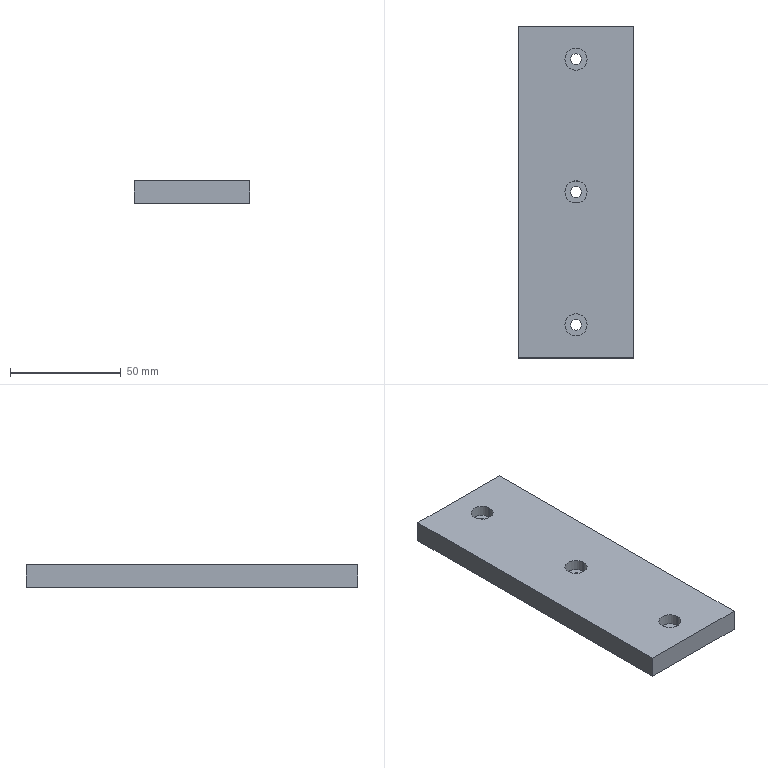Part | SolidWorks | features Chamfer 1, Extrusion 1, HoleWzd 1 | 1 solid | 21 faces | box 52 x 150 x 10 mm | volume 76527 mm3 | cylinder 12 | plane 9 | commonest cylinder face diameters 5 x6 10 x6
STEP:
#1=CARTESIAN_POINT('',(-5.,60.,0.));
#2=VERTEX_POINT('',#1);
#3=CARTESIAN_POINT('',(5.,60.,0.));
#4=VERTEX_POINT('',#3);
#5=CARTESIAN_POINT('',(0.,60.,0.));
#6=DIRECTION('',(0.,0.,1.));
#7=DIRECTION('',(1.,0.,0.));
#8=AXIS2_PLACEMENT_3D('',#5,#6,#7);
#9=CIRCLE('',#8,5.);
#10=EDGE_CURVE('',#2,#4,#9,.T.);
#11=ORIENTED_EDGE('',*,*,#10,.F.);
#12=CARTESIAN_POINT('',(-5.,60.,5.));
#13=VERTEX_POINT('',#12);
#14=CARTESIAN_POINT('',(-5.,60.,5.));
#15=DIRECTION('',(0.,0.,1.));
#16=VECTOR('',#15,1000.);
#17=LINE('',#14,#16);
#18=EDGE_CURVE('',#2,#13,#17,.T.);
#19=ORIENTED_EDGE('',*,*,#18,.T.);
#20=CARTESIAN_POINT('',(5.,60.,5.));
#21=VERTEX_POINT('',#20);
#22=CARTESIAN_POINT('',(0.,60.,5.));
#23=DIRECTION('',(0.,0.,1.));
#24=DIRECTION('',(1.,0.,0.));
#25=AXIS2_PLACEMENT_3D('',#22,#23,#24);
#26=CIRCLE('',#25,5.);
#27=EDGE_CURVE('',#13,#21,#26,.T.);
#28=ORIENTED_EDGE('',*,*,#27,.T.);
#29=CARTESIAN_POINT('',(5.,60.,5.));
#30=DIRECTION('',(0.,0.,1.));
#31=VECTOR('',#30,1000.);
#32=LINE('',#29,#31);
#33=EDGE_CURVE('',#4,#21,#32,.T.);
#34=ORIENTED_EDGE('',*,*,#33,.F.);
#35=EDGE_LOOP('',(#11,#19,#28,#34));
#36=FACE_OUTER_BOUND('',#35,.T.);
#37=CARTESIAN_POINT('',(0.,60.,5.));
#38=DIRECTION('',(0.,0.,1.));
#39=DIRECTION('',(1.,0.,0.));
#40=AXIS2_PLACEMENT_3D('',#37,#38,#39);
#41=CYLINDRICAL_SURFACE('',#40,5.);
#42=ADVANCED_FACE('',(#36),#41,.F.);
#43=CARTESIAN_POINT('',(-2.5,60.,-5.));
#44=VERTEX_POINT('',#43);
#45=CARTESIAN_POINT('',(2.5,60.,-5.));
#46=VERTEX_POINT('',#45);
#47=CARTESIAN_POINT('',(0.,60.,-5.));
#48=DIRECTION('',(0.,0.,1.));
#49=DIRECTION('',(1.,0.,0.));
#50=AXIS2_PLACEMENT_3D('',#47,#48,#49);
#51=CIRCLE('',#50,2.5);
#52=EDGE_CURVE('',#44,#46,#51,.T.);
#53=ORIENTED_EDGE('',*,*,#52,.F.);
#54=CARTESIAN_POINT('',(-2.5,60.,0.));
#55=VERTEX_POINT('',#54);
#56=CARTESIAN_POINT('',(-2.5,60.,5.));
#57=DIRECTION('',(0.,0.,1.));
#58=VECTOR('',#57,1000.);
#59=LINE('',#56,#58);
#60=EDGE_CURVE('',#44,#55,#59,.T.);
#61=ORIENTED_EDGE('',*,*,#60,.T.);
#62=CARTESIAN_POINT('',(2.5,60.,0.));
#63=VERTEX_POINT('',#62);
#64=CARTESIAN_POINT('',(0.,60.,0.));
#65=DIRECTION('',(0.,0.,1.));
#66=DIRECTION('',(1.,0.,0.));
#67=AXIS2_PLACEMENT_3D('',#64,#65,#66);
#68=CIRCLE('',#67,2.5);
#69=EDGE_CURVE('',#55,#63,#68,.T.);
#70=ORIENTED_EDGE('',*,*,#69,.T.);
#71=CARTESIAN_POINT('',(2.5,60.,5.));
#72=DIRECTION('',(0.,0.,1.));
#73=VECTOR('',#72,1000.);
#74=LINE('',#71,#73);
#75=EDGE_CURVE('',#46,#63,#74,.T.);
#76=ORIENTED_EDGE('',*,*,#75,.F.);
#77=EDGE_LOOP('',(#53,#61,#70,#76));
#78=FACE_OUTER_BOUND('',#77,.T.);
#79=CARTESIAN_POINT('',(0.,60.,5.));
#80=DIRECTION('',(0.,0.,1.));
#81=DIRECTION('',(1.,0.,0.));
#82=AXIS2_PLACEMENT_3D('',#79,#80,#81);
#83=CYLINDRICAL_SURFACE('',#82,2.5);
#84=ADVANCED_FACE('',(#78),#83,.F.);
#85=CARTESIAN_POINT('',(-5.,-60.,0.));
#86=VERTEX_POINT('',#85);
#87=CARTESIAN_POINT('',(5.,-60.,0.));
#88=VERTEX_POINT('',#87);
#89=CARTESIAN_POINT('',(0.,-60.,0.));
#90=DIRECTION('',(0.,0.,1.));
#91=DIRECTION('',(1.,0.,0.));
#92=AXIS2_PLACEMENT_3D('',#89,#90,#91);
#93=CIRCLE('',#92,5.);
#94=EDGE_CURVE('',#86,#88,#93,.T.);
#95=ORIENTED_EDGE('',*,*,#94,.F.);
#96=CARTESIAN_POINT('',(-5.,-60.,5.));
#97=VERTEX_POINT('',#96);
#98=CARTESIAN_POINT('',(-5.,-60.,5.));
#99=DIRECTION('',(0.,0.,1.));
#100=VECTOR('',#99,1000.);
#101=LINE('',#98,#100);
#102=EDGE_CURVE('',#86,#97,#101,.T.);
#103=ORIENTED_EDGE('',*,*,#102,.T.);
#104=CARTESIAN_POINT('',(5.,-60.,5.));
#105=VERTEX_POINT('',#104);
#106=CARTESIAN_POINT('',(0.,-60.,5.));
#107=DIRECTION('',(0.,0.,1.));
#108=DIRECTION('',(1.,0.,0.));
#109=AXIS2_PLACEMENT_3D('',#106,#107,#108);
#110=CIRCLE('',#109,5.);
#111=EDGE_CURVE('',#97,#105,#110,.T.);
#112=ORIENTED_EDGE('',*,*,#111,.T.);
#113=CARTESIAN_POINT('',(5.,-60.,5.));
#114=DIRECTION('',(0.,0.,1.));
#115=VECTOR('',#114,1000.);
#116=LINE('',#113,#115);
#117=EDGE_CURVE('',#88,#105,#116,.T.);
#118=ORIENTED_EDGE('',*,*,#117,.F.);
#119=EDGE_LOOP('',(#95,#103,#112,#118));
#120=FACE_OUTER_BOUND('',#119,.T.);
#121=CARTESIAN_POINT('',(0.,-60.,5.));
#122=DIRECTION('',(0.,0.,1.));
#123=DIRECTION('',(1.,0.,0.));
#124=AXIS2_PLACEMENT_3D('',#121,#122,#123);
#125=CYLINDRICAL_SURFACE('',#124,5.);
#126=ADVANCED_FACE('',(#120),#125,.F.);
#127=CARTESIAN_POINT('',(-2.5,-60.,-5.));
#128=VERTEX_POINT('',#127);
#129=CARTESIAN_POINT('',(2.5,-60.,-5.));
#130=VERTEX_POINT('',#129);
#131=CARTESIAN_POINT('',(0.,-60.,-5.));
#132=DIRECTION('',(0.,0.,1.));
#133=DIRECTION('',(1.,0.,0.));
#134=AXIS2_PLACEMENT_3D('',#131,#132,#133);
#135=CIRCLE('',#134,2.5);
#136=EDGE_CURVE('',#128,#130,#135,.T.);
#137=ORIENTED_EDGE('',*,*,#136,.F.);
#138=CARTESIAN_POINT('',(-2.5,-60.,0.));
#139=VERTEX_POINT('',#138);
#140=CARTESIAN_POINT('',(-2.5,-60.,5.));
#141=DIRECTION('',(0.,0.,1.));
#142=VECTOR('',#141,1000.);
#143=LINE('',#140,#142);
#144=EDGE_CURVE('',#128,#139,#143,.T.);
#145=ORIENTED_EDGE('',*,*,#144,.T.);
#146=CARTESIAN_POINT('',(2.5,-60.,0.));
#147=VERTEX_POINT('',#146);
#148=CARTESIAN_POINT('',(0.,-60.,0.));
#149=DIRECTION('',(0.,0.,1.));
#150=DIRECTION('',(1.,0.,0.));
#151=AXIS2_PLACEMENT_3D('',#148,#149,#150);
#152=CIRCLE('',#151,2.5);
#153=EDGE_CURVE('',#139,#147,#152,.T.);
#154=ORIENTED_EDGE('',*,*,#153,.T.);
#155=CARTESIAN_POINT('',(2.5,-60.,5.));
#156=DIRECTION('',(0.,0.,1.));
#157=VECTOR('',#156,1000.);
#158=LINE('',#155,#157);
#159=EDGE_CURVE('',#130,#147,#158,.T.);
#160=ORIENTED_EDGE('',*,*,#159,.F.);
#161=EDGE_LOOP('',(#137,#145,#154,#160));
#162=FACE_OUTER_BOUND('',#161,.T.);
#163=CARTESIAN_POINT('',(0.,-60.,5.));
#164=DIRECTION('',(0.,0.,1.));
#165=DIRECTION('',(1.,0.,0.));
#166=AXIS2_PLACEMENT_3D('',#163,#164,#165);
#167=CYLINDRICAL_SURFACE('',#166,2.5);
#168=ADVANCED_FACE('',(#162),#167,.F.);
#169=CARTESIAN_POINT('',(-5.,0.,0.));
#170=VERTEX_POINT('',#169);
#171=CARTESIAN_POINT('',(5.,0.,0.));
#172=VERTEX_POINT('',#171);
#173=CARTESIAN_POINT('',(0.,0.,0.));
#174=DIRECTION('',(0.,0.,1.));
#175=DIRECTION('',(1.,0.,0.));
#176=AXIS2_PLACEMENT_3D('',#173,#174,#175);
#177=CIRCLE('',#176,5.);
#178=EDGE_CURVE('',#170,#172,#177,.T.);
#179=ORIENTED_EDGE('',*,*,#178,.F.);
#180=CARTESIAN_POINT('',(-5.,0.,5.));
#181=VERTEX_POINT('',#180);
#182=CARTESIAN_POINT('',(-5.,0.,5.));
#183=DIRECTION('',(0.,0.,1.));
#184=VECTOR('',#183,1000.);
#185=LINE('',#182,#184);
#186=EDGE_CURVE('',#170,#181,#185,.T.);
#187=ORIENTED_EDGE('',*,*,#186,.T.);
#188=CARTESIAN_POINT('',(5.,0.,5.));
#189=VERTEX_POINT('',#188);
#190=CARTESIAN_POINT('',(0.,0.,5.));
#191=DIRECTION('',(0.,0.,1.));
#192=DIRECTION('',(1.,0.,0.));
#193=AXIS2_PLACEMENT_3D('',#190,#191,#192);
#194=CIRCLE('',#193,5.);
#195=EDGE_CURVE('',#181,#189,#194,.T.);
#196=ORIENTED_EDGE('',*,*,#195,.T.);
#197=CARTESIAN_POINT('',(5.,0.,5.));
#198=DIRECTION('',(0.,0.,1.));
#199=VECTOR('',#198,1000.);
#200=LINE('',#197,#199);
#201=EDGE_CURVE('',#172,#189,#200,.T.);
#202=ORIENTED_EDGE('',*,*,#201,.F.);
#203=EDGE_LOOP('',(#179,#187,#196,#202));
#204=FACE_OUTER_BOUND('',#203,.T.);
#205=CARTESIAN_POINT('',(0.,0.,5.));
#206=DIRECTION('',(0.,0.,1.));
#207=DIRECTION('',(1.,0.,0.));
#208=AXIS2_PLACEMENT_3D('',#205,#206,#207);
#209=CYLINDRICAL_SURFACE('',#208,5.);
#210=ADVANCED_FACE('',(#204),#209,.F.);
#211=CARTESIAN_POINT('',(-2.5,0.,-5.));
#212=VERTEX_POINT('',#211);
#213=CARTESIAN_POINT('',(2.5,0.,-5.));
#214=VERTEX_POINT('',#213);
#215=CARTESIAN_POINT('',(0.,0.,-5.));
#216=DIRECTION('',(0.,0.,1.));
#217=DIRECTION('',(1.,0.,0.));
#218=AXIS2_PLACEMENT_3D('',#215,#216,#217);
#219=CIRCLE('',#218,2.5);
#220=EDGE_CURVE('',#212,#214,#219,.T.);
#221=ORIENTED_EDGE('',*,*,#220,.F.);
#222=CARTESIAN_POINT('',(-2.5,0.,0.));
#223=VERTEX_POINT('',#222);
#224=CARTESIAN_POINT('',(-2.5,0.,5.));
#225=DIRECTION('',(0.,0.,1.));
#226=VECTOR('',#225,1000.);
#227=LINE('',#224,#226);
#228=EDGE_CURVE('',#212,#223,#227,.T.);
#229=ORIENTED_EDGE('',*,*,#228,.T.);
#230=CARTESIAN_POINT('',(2.5,0.,0.));
#231=VERTEX_POINT('',#230);
#232=CARTESIAN_POINT('',(0.,0.,0.));
#233=DIRECTION('',(0.,0.,1.));
#234=DIRECTION('',(1.,0.,0.));
#235=AXIS2_PLACEMENT_3D('',#232,#233,#234);
#236=CIRCLE('',#235,2.5);
#237=EDGE_CURVE('',#223,#231,#236,.T.);
#238=ORIENTED_EDGE('',*,*,#237,.T.);
#239=CARTESIAN_POINT('',(2.5,0.,5.));
#240=DIRECTION('',(0.,0.,1.));
#241=VECTOR('',#240,1000.);
#242=LINE('',#239,#241);
#243=EDGE_CURVE('',#214,#231,#242,.T.);
#244=ORIENTED_EDGE('',*,*,#243,.F.);
#245=EDGE_LOOP('',(#221,#229,#238,#244));
#246=FACE_OUTER_BOUND('',#245,.T.);
#247=CARTESIAN_POINT('',(0.,0.,5.));
#248=DIRECTION('',(0.,0.,1.));
#249=DIRECTION('',(1.,0.,0.));
#250=AXIS2_PLACEMENT_3D('',#247,#248,#249);
#251=CYLINDRICAL_SURFACE('',#250,2.5);
#252=ADVANCED_FACE('',(#246),#251,.F.);
#253=CARTESIAN_POINT('',(-26.,75.,-5.));
#254=VERTEX_POINT('',#253);
#255=CARTESIAN_POINT('',(-26.,-75.,-5.));
#256=VERTEX_POINT('',#255);
#257=CARTESIAN_POINT('',(-26.,-75.,-5.));
#258=DIRECTION('',(0.,-1.,0.));
#259=VECTOR('',#258,1000.);
#260=LINE('',#257,#259);
#261=EDGE_CURVE('',#254,#256,#260,.T.);
#262=ORIENTED_EDGE('',*,*,#261,.T.);
#263=CARTESIAN_POINT('',(-26.,-75.,5.));
#264=VERTEX_POINT('',#263);
#265=CARTESIAN_POINT('',(-26.,-75.,5.));
#266=DIRECTION('',(0.,0.,-1.));
#267=VECTOR('',#266,1000.);
#268=LINE('',#265,#267);
#269=EDGE_CURVE('',#264,#256,#268,.T.);
#270=ORIENTED_EDGE('',*,*,#269,.F.);
#271=CARTESIAN_POINT('',(-26.,75.,5.));
#272=VERTEX_POINT('',#271);
#273=CARTESIAN_POINT('',(-26.,-75.,5.));
#274=DIRECTION('',(0.,-1.,0.));
#275=VECTOR('',#274,1000.);
#276=LINE('',#273,#275);
#277=EDGE_CURVE('',#272,#264,#276,.T.);
#278=ORIENTED_EDGE('',*,*,#277,.F.);
#279=CARTESIAN_POINT('',(-26.,75.,5.));
#280=DIRECTION('',(0.,0.,-1.));
#281=VECTOR('',#280,1000.);
#282=LINE('',#279,#281);
#283=EDGE_CURVE('',#272,#254,#282,.T.);
#284=ORIENTED_EDGE('',*,*,#283,.T.);
#285=EDGE_LOOP('',(#262,#270,#278,#284));
#286=FACE_OUTER_BOUND('',#285,.T.);
#287=CARTESIAN_POINT('',(-26.,-75.,5.));
#288=DIRECTION('',(1.,0.,0.));
#289=DIRECTION('',(0.,0.,-1.));
#290=AXIS2_PLACEMENT_3D('',#287,#288,#289);
#291=PLANE('',#290);
#292=ADVANCED_FACE('',(#286),#291,.F.);
#293=CARTESIAN_POINT('',(26.,-75.,-5.));
#294=VERTEX_POINT('',#293);
#295=CARTESIAN_POINT('',(26.,-75.,-5.));
#296=DIRECTION('',(1.,0.,0.));
#297=VECTOR('',#296,1000.);
#298=LINE('',#295,#297);
#299=EDGE_CURVE('',#256,#294,#298,.T.);
#300=ORIENTED_EDGE('',*,*,#299,.T.);
#301=CARTESIAN_POINT('',(26.,-75.,5.));
#302=VERTEX_POINT('',#301);
#303=CARTESIAN_POINT('',(26.,-75.,5.));
#304=DIRECTION('',(0.,0.,-1.));
#305=VECTOR('',#304,1000.);
#306=LINE('',#303,#305);
#307=EDGE_CURVE('',#302,#294,#306,.T.);
#308=ORIENTED_EDGE('',*,*,#307,.F.);
#309=CARTESIAN_POINT('',(26.,-75.,5.));
#310=DIRECTION('',(1.,0.,0.));
#311=VECTOR('',#310,1000.);
#312=LINE('',#309,#311);
#313=EDGE_CURVE('',#264,#302,#312,.T.);
#314=ORIENTED_EDGE('',*,*,#313,.F.);
#315=ORIENTED_EDGE('',*,*,#269,.T.);
#316=EDGE_LOOP('',(#300,#308,#314,#315));
#317=FACE_OUTER_BOUND('',#316,.T.);
#318=CARTESIAN_POINT('',(26.,-75.,5.));
#319=DIRECTION('',(0.,1.,0.));
#320=DIRECTION('',(0.,0.,1.));
#321=AXIS2_PLACEMENT_3D('',#318,#319,#320);
#322=PLANE('',#321);
#323=ADVANCED_FACE('',(#317),#322,.F.);
#324=CARTESIAN_POINT('',(26.,75.,-5.));
#325=VERTEX_POINT('',#324);
#326=CARTESIAN_POINT('',(26.,-75.,-5.));
#327=DIRECTION('',(0.,1.,0.));
#328=VECTOR('',#327,1000.);
#329=LINE('',#326,#328);
#330=EDGE_CURVE('',#294,#325,#329,.T.);
#331=ORIENTED_EDGE('',*,*,#330,.T.);
#332=CARTESIAN_POINT('',(26.,75.,5.));
#333=VERTEX_POINT('',#332);
#334=CARTESIAN_POINT('',(26.,75.,5.));
#335=DIRECTION('',(0.,0.,-1.));
#336=VECTOR('',#335,1000.);
#337=LINE('',#334,#336);
#338=EDGE_CURVE('',#333,#325,#337,.T.);
#339=ORIENTED_EDGE('',*,*,#338,.F.);
#340=CARTESIAN_POINT('',(26.,-75.,5.));
#341=DIRECTION('',(0.,1.,0.));
#342=VECTOR('',#341,1000.);
#343=LINE('',#340,#342);
#344=EDGE_CURVE('',#302,#333,#343,.T.);
#345=ORIENTED_EDGE('',*,*,#344,.F.);
#346=ORIENTED_EDGE('',*,*,#307,.T.);
#347=EDGE_LOOP('',(#331,#339,#345,#346));
#348=FACE_OUTER_BOUND('',#347,.T.);
#349=CARTESIAN_POINT('',(26.,-75.,5.));
#350=DIRECTION('',(-1.,0.,0.));
#351=DIRECTION('',(0.,0.,1.));
#352=AXIS2_PLACEMENT_3D('',#349,#350,#351);
#353=PLANE('',#352);
#354=ADVANCED_FACE('',(#348),#353,.F.);
#355=CARTESIAN_POINT('',(26.,75.,-5.));
#356=DIRECTION('',(-1.,0.,0.));
#357=VECTOR('',#356,1000.);
#358=LINE('',#355,#357);
#359=EDGE_CURVE('',#325,#254,#358,.T.);
#360=ORIENTED_EDGE('',*,*,#359,.T.);
#361=ORIENTED_EDGE('',*,*,#283,.F.);
#362=CARTESIAN_POINT('',(26.,75.,5.));
#363=DIRECTION('',(-1.,0.,0.));
#364=VECTOR('',#363,1000.);
#365=LINE('',#362,#364);
#366=EDGE_CURVE('',#333,#272,#365,.T.);
#367=ORIENTED_EDGE('',*,*,#366,.F.);
#368=ORIENTED_EDGE('',*,*,#338,.T.);
#369=EDGE_LOOP('',(#360,#361,#367,#368));
#370=FACE_OUTER_BOUND('',#369,.T.);
#371=CARTESIAN_POINT('',(26.,75.,5.));
#372=DIRECTION('',(0.,-1.,0.));
#373=DIRECTION('',(0.,0.,-1.));
#374=AXIS2_PLACEMENT_3D('',#371,#372,#373);
#375=PLANE('',#374);
#376=ADVANCED_FACE('',(#370),#375,.F.);
#377=CARTESIAN_POINT('',(0.,60.,5.));
#378=DIRECTION('',(0.,0.,1.));
#379=DIRECTION('',(1.,0.,0.));
#380=AXIS2_PLACEMENT_3D('',#377,#378,#379);
#381=CIRCLE('',#380,5.);
#382=EDGE_CURVE('',#21,#13,#381,.T.);
#383=ORIENTED_EDGE('',*,*,#382,.F.);
#384=ORIENTED_EDGE('',*,*,#27,.F.);
#385=EDGE_LOOP('',(#383,#384));
#386=FACE_BOUND('',#385,.T.);
#387=CARTESIAN_POINT('',(0.,-60.,5.));
#388=DIRECTION('',(0.,0.,1.));
#389=DIRECTION('',(1.,0.,0.));
#390=AXIS2_PLACEMENT_3D('',#387,#388,#389);
#391=CIRCLE('',#390,5.);
#392=EDGE_CURVE('',#105,#97,#391,.T.);
#393=ORIENTED_EDGE('',*,*,#392,.F.);
#394=ORIENTED_EDGE('',*,*,#111,.F.);
#395=EDGE_LOOP('',(#393,#394));
#396=FACE_BOUND('',#395,.T.);
#397=CARTESIAN_POINT('',(0.,0.,5.));
#398=DIRECTION('',(0.,0.,1.));
#399=DIRECTION('',(1.,0.,0.));
#400=AXIS2_PLACEMENT_3D('',#397,#398,#399);
#401=CIRCLE('',#400,5.);
#402=EDGE_CURVE('',#189,#181,#401,.T.);
#403=ORIENTED_EDGE('',*,*,#402,.F.);
#404=ORIENTED_EDGE('',*,*,#195,.F.);
#405=EDGE_LOOP('',(#403,#404));
#406=FACE_BOUND('',#405,.T.);
#407=ORIENTED_EDGE('',*,*,#277,.T.);
#408=ORIENTED_EDGE('',*,*,#313,.T.);
#409=ORIENTED_EDGE('',*,*,#344,.T.);
#410=ORIENTED_EDGE('',*,*,#366,.T.);
#411=EDGE_LOOP('',(#407,#408,#409,#410));
#412=FACE_OUTER_BOUND('',#411,.T.);
#413=CARTESIAN_POINT('',(0.,0.,5.));
#414=DIRECTION('',(0.,0.,1.));
#415=DIRECTION('',(1.,0.,0.));
#416=AXIS2_PLACEMENT_3D('',#413,#414,#415);
#417=PLANE('',#416);
#418=ADVANCED_FACE('',(#386,#396,#406,#412),#417,.T.);
#419=CARTESIAN_POINT('',(0.,60.,-5.));
#420=DIRECTION('',(0.,0.,1.));
#421=DIRECTION('',(1.,0.,0.));
#422=AXIS2_PLACEMENT_3D('',#419,#420,#421);
#423=CIRCLE('',#422,2.5);
#424=EDGE_CURVE('',#46,#44,#423,.T.);
#425=ORIENTED_EDGE('',*,*,#424,.T.);
#426=ORIENTED_EDGE('',*,*,#52,.T.);
#427=EDGE_LOOP('',(#425,#426));
#428=FACE_BOUND('',#427,.T.);
#429=CARTESIAN_POINT('',(0.,-60.,-5.));
#430=DIRECTION('',(0.,0.,1.));
#431=DIRECTION('',(1.,0.,0.));
#432=AXIS2_PLACEMENT_3D('',#429,#430,#431);
#433=CIRCLE('',#432,2.5);
#434=EDGE_CURVE('',#130,#128,#433,.T.);
#435=ORIENTED_EDGE('',*,*,#434,.T.);
#436=ORIENTED_EDGE('',*,*,#136,.T.);
#437=EDGE_LOOP('',(#435,#436));
#438=FACE_BOUND('',#437,.T.);
#439=CARTESIAN_POINT('',(0.,0.,-5.));
#440=DIRECTION('',(0.,0.,1.));
#441=DIRECTION('',(1.,0.,0.));
#442=AXIS2_PLACEMENT_3D('',#439,#440,#441);
#443=CIRCLE('',#442,2.5);
#444=EDGE_CURVE('',#214,#212,#443,.T.);
#445=ORIENTED_EDGE('',*,*,#444,.T.);
#446=ORIENTED_EDGE('',*,*,#220,.T.);
#447=EDGE_LOOP('',(#445,#446));
#448=FACE_BOUND('',#447,.T.);
#449=ORIENTED_EDGE('',*,*,#261,.F.);
#450=ORIENTED_EDGE('',*,*,#359,.F.);
#451=ORIENTED_EDGE('',*,*,#330,.F.);
#452=ORIENTED_EDGE('',*,*,#299,.F.);
#453=EDGE_LOOP('',(#449,#450,#451,#452));
#454=FACE_OUTER_BOUND('',#453,.T.);
#455=CARTESIAN_POINT('',(0.,0.,-5.));
#456=DIRECTION('',(0.,0.,1.));
#457=DIRECTION('',(1.,0.,0.));
#458=AXIS2_PLACEMENT_3D('',#455,#456,#457);
#459=PLANE('',#458);
#460=ADVANCED_FACE('',(#428,#438,#448,#454),#459,.F.);
#461=ORIENTED_EDGE('',*,*,#228,.F.);
#462=ORIENTED_EDGE('',*,*,#444,.F.);
#463=ORIENTED_EDGE('',*,*,#243,.T.);
#464=CARTESIAN_POINT('',(0.,0.,0.));
#465=DIRECTION('',(0.,0.,1.));
#466=DIRECTION('',(1.,0.,0.));
#467=AXIS2_PLACEMENT_3D('',#464,#465,#466);
#468=CIRCLE('',#467,2.5);
#469=EDGE_CURVE('',#231,#223,#468,.T.);
#470=ORIENTED_EDGE('',*,*,#469,.T.);
#471=EDGE_LOOP('',(#461,#462,#463,#470));
#472=FACE_OUTER_BOUND('',#471,.T.);
#473=CARTESIAN_POINT('',(0.,0.,5.));
#474=DIRECTION('',(0.,0.,1.));
#475=DIRECTION('',(1.,0.,0.));
#476=AXIS2_PLACEMENT_3D('',#473,#474,#475);
#477=CYLINDRICAL_SURFACE('',#476,2.5);
#478=ADVANCED_FACE('',(#472),#477,.F.);
#479=ORIENTED_EDGE('',*,*,#469,.F.);
#480=ORIENTED_EDGE('',*,*,#237,.F.);
#481=EDGE_LOOP('',(#479,#480));
#482=FACE_BOUND('',#481,.T.);
#483=CARTESIAN_POINT('',(0.,0.,0.));
#484=DIRECTION('',(0.,0.,1.));
#485=DIRECTION('',(1.,0.,0.));
#486=AXIS2_PLACEMENT_3D('',#483,#484,#485);
#487=CIRCLE('',#486,5.);
#488=EDGE_CURVE('',#172,#170,#487,.T.);
#489=ORIENTED_EDGE('',*,*,#488,.T.);
#490=ORIENTED_EDGE('',*,*,#178,.T.);
#491=EDGE_LOOP('',(#489,#490));
#492=FACE_OUTER_BOUND('',#491,.T.);
#493=CARTESIAN_POINT('',(2.5,0.,0.));
#494=DIRECTION('',(0.,0.,-1.));
#495=DIRECTION('',(-1.,0.,0.));
#496=AXIS2_PLACEMENT_3D('',#493,#494,#495);
#497=PLANE('',#496);
#498=ADVANCED_FACE('',(#482,#492),#497,.F.);
#499=ORIENTED_EDGE('',*,*,#186,.F.);
#500=ORIENTED_EDGE('',*,*,#488,.F.);
#501=ORIENTED_EDGE('',*,*,#201,.T.);
#502=ORIENTED_EDGE('',*,*,#402,.T.);
#503=EDGE_LOOP('',(#499,#500,#501,#502));
#504=FACE_OUTER_BOUND('',#503,.T.);
#505=CARTESIAN_POINT('',(0.,0.,5.));
#506=DIRECTION('',(0.,0.,1.));
#507=DIRECTION('',(1.,0.,0.));
#508=AXIS2_PLACEMENT_3D('',#505,#506,#507);
#509=CYLINDRICAL_SURFACE('',#508,5.);
#510=ADVANCED_FACE('',(#504),#509,.F.);
#511=ORIENTED_EDGE('',*,*,#144,.F.);
#512=ORIENTED_EDGE('',*,*,#434,.F.);
#513=ORIENTED_EDGE('',*,*,#159,.T.);
#514=CARTESIAN_POINT('',(0.,-60.,0.));
#515=DIRECTION('',(0.,0.,1.));
#516=DIRECTION('',(1.,0.,0.));
#517=AXIS2_PLACEMENT_3D('',#514,#515,#516);
#518=CIRCLE('',#517,2.5);
#519=EDGE_CURVE('',#147,#139,#518,.T.);
#520=ORIENTED_EDGE('',*,*,#519,.T.);
#521=EDGE_LOOP('',(#511,#512,#513,#520));
#522=FACE_OUTER_BOUND('',#521,.T.);
#523=CARTESIAN_POINT('',(0.,-60.,5.));
#524=DIRECTION('',(0.,0.,1.));
#525=DIRECTION('',(1.,0.,0.));
#526=AXIS2_PLACEMENT_3D('',#523,#524,#525);
#527=CYLINDRICAL_SURFACE('',#526,2.5);
#528=ADVANCED_FACE('',(#522),#527,.F.);
#529=ORIENTED_EDGE('',*,*,#519,.F.);
#530=ORIENTED_EDGE('',*,*,#153,.F.);
#531=EDGE_LOOP('',(#529,#530));
#532=FACE_BOUND('',#531,.T.);
#533=CARTESIAN_POINT('',(0.,-60.,0.));
#534=DIRECTION('',(0.,0.,1.));
#535=DIRECTION('',(1.,0.,0.));
#536=AXIS2_PLACEMENT_3D('',#533,#534,#535);
#537=CIRCLE('',#536,5.);
#538=EDGE_CURVE('',#88,#86,#537,.T.);
#539=ORIENTED_EDGE('',*,*,#538,.T.);
#540=ORIENTED_EDGE('',*,*,#94,.T.);
#541=EDGE_LOOP('',(#539,#540));
#542=FACE_OUTER_BOUND('',#541,.T.);
#543=CARTESIAN_POINT('',(2.5,-60.,0.));
#544=DIRECTION('',(0.,0.,-1.));
#545=DIRECTION('',(-1.,0.,0.));
#546=AXIS2_PLACEMENT_3D('',#543,#544,#545);
#547=PLANE('',#546);
#548=ADVANCED_FACE('',(#532,#542),#547,.F.);
#549=ORIENTED_EDGE('',*,*,#102,.F.);
#550=ORIENTED_EDGE('',*,*,#538,.F.);
#551=ORIENTED_EDGE('',*,*,#117,.T.);
#552=ORIENTED_EDGE('',*,*,#392,.T.);
#553=EDGE_LOOP('',(#549,#550,#551,#552));
#554=FACE_OUTER_BOUND('',#553,.T.);
#555=CARTESIAN_POINT('',(0.,-60.,5.));
#556=DIRECTION('',(0.,0.,1.));
#557=DIRECTION('',(1.,0.,0.));
#558=AXIS2_PLACEMENT_3D('',#555,#556,#557);
#559=CYLINDRICAL_SURFACE('',#558,5.);
#560=ADVANCED_FACE('',(#554),#559,.F.);
#561=ORIENTED_EDGE('',*,*,#60,.F.);
#562=ORIENTED_EDGE('',*,*,#424,.F.);
#563=ORIENTED_EDGE('',*,*,#75,.T.);
#564=CARTESIAN_POINT('',(0.,60.,0.));
#565=DIRECTION('',(0.,0.,1.));
#566=DIRECTION('',(1.,0.,0.));
#567=AXIS2_PLACEMENT_3D('',#564,#565,#566);
#568=CIRCLE('',#567,2.5);
#569=EDGE_CURVE('',#63,#55,#568,.T.);
#570=ORIENTED_EDGE('',*,*,#569,.T.);
#571=EDGE_LOOP('',(#561,#562,#563,#570));
#572=FACE_OUTER_BOUND('',#571,.T.);
#573=CARTESIAN_POINT('',(0.,60.,5.));
#574=DIRECTION('',(0.,0.,1.));
#575=DIRECTION('',(1.,0.,0.));
#576=AXIS2_PLACEMENT_3D('',#573,#574,#575);
#577=CYLINDRICAL_SURFACE('',#576,2.5);
#578=ADVANCED_FACE('',(#572),#577,.F.);
#579=ORIENTED_EDGE('',*,*,#569,.F.);
#580=ORIENTED_EDGE('',*,*,#69,.F.);
#581=EDGE_LOOP('',(#579,#580));
#582=FACE_BOUND('',#581,.T.);
#583=CARTESIAN_POINT('',(0.,60.,0.));
#584=DIRECTION('',(0.,0.,1.));
#585=DIRECTION('',(1.,0.,0.));
#586=AXIS2_PLACEMENT_3D('',#583,#584,#585);
#587=CIRCLE('',#586,5.);
#588=EDGE_CURVE('',#4,#2,#587,.T.);
#589=ORIENTED_EDGE('',*,*,#588,.T.);
#590=ORIENTED_EDGE('',*,*,#10,.T.);
#591=EDGE_LOOP('',(#589,#590));
#592=FACE_OUTER_BOUND('',#591,.T.);
#593=CARTESIAN_POINT('',(2.5,60.,0.));
#594=DIRECTION('',(0.,0.,-1.));
#595=DIRECTION('',(-1.,0.,0.));
#596=AXIS2_PLACEMENT_3D('',#593,#594,#595);
#597=PLANE('',#596);
#598=ADVANCED_FACE('',(#582,#592),#597,.F.);
#599=ORIENTED_EDGE('',*,*,#18,.F.);
#600=ORIENTED_EDGE('',*,*,#588,.F.);
#601=ORIENTED_EDGE('',*,*,#33,.T.);
#602=ORIENTED_EDGE('',*,*,#382,.T.);
#603=EDGE_LOOP('',(#599,#600,#601,#602));
#604=FACE_OUTER_BOUND('',#603,.T.);
#605=CARTESIAN_POINT('',(0.,60.,5.));
#606=DIRECTION('',(0.,0.,1.));
#607=DIRECTION('',(1.,0.,0.));
#608=AXIS2_PLACEMENT_3D('',#605,#606,#607);
#609=CYLINDRICAL_SURFACE('',#608,5.);
#610=ADVANCED_FACE('',(#604),#609,.F.);
#611=CLOSED_SHELL('',(#42,#84,#126,#168,#210,#252,#292,#323,#354,#376,#418,#460,#478,#498,#510,#528,#548,#560,#578,#598,#610));
#612=MANIFOLD_SOLID_BREP('',#611);
#613=CARTESIAN_POINT('',(0.,0.,0.));
#614=DIRECTION('',(0.,0.,1.));
#615=DIRECTION('',(1.,0.,0.));
#616=AXIS2_PLACEMENT_3D('',#613,#614,#615);
#617=(LENGTH_UNIT()NAMED_UNIT(*)SI_UNIT(.MILLI.,.METRE.));
#618=UNCERTAINTY_MEASURE_WITH_UNIT(LENGTH_MEASURE(0.00001),#617,'','');
#619=(NAMED_UNIT(*)PLANE_ANGLE_UNIT()SI_UNIT($,.RADIAN.));
#620=(NAMED_UNIT(*)SI_UNIT($,.STERADIAN.)SOLID_ANGLE_UNIT());
#621=(GEOMETRIC_REPRESENTATION_CONTEXT(3)GLOBAL_UNCERTAINTY_ASSIGNED_CONTEXT((#618))GLOBAL_UNIT_ASSIGNED_CONTEXT((#617,#619,#620))REPRESENTATION_CONTEXT('',''));
#622=ADVANCED_BREP_SHAPE_REPRESENTATION('',(#612,#616),#621);